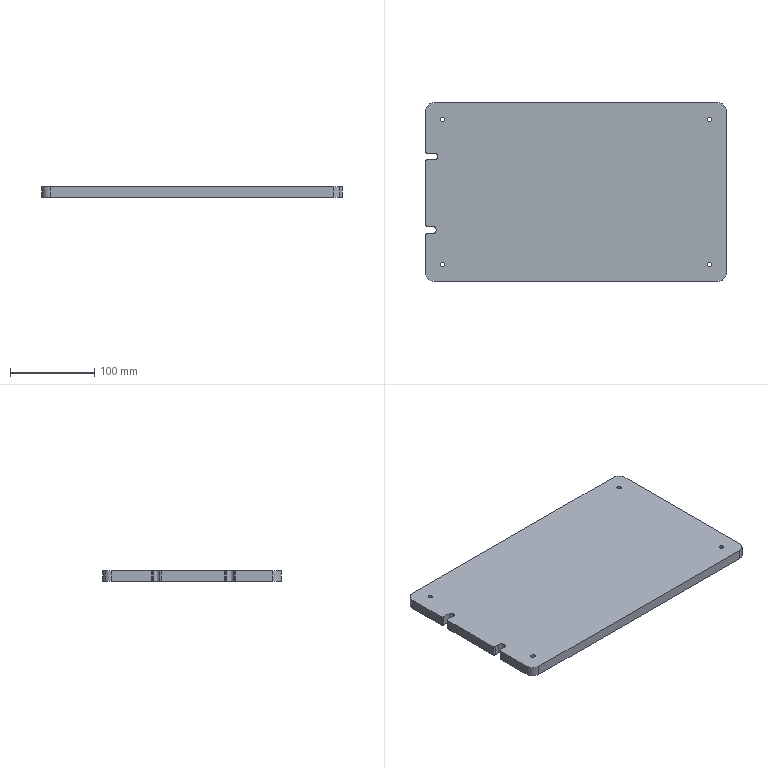Part | STEP file | ASND-0110-6.2aq | 1 solid | 49 faces | box 357.093 x 212.456 x 12 mm | volume 877711 mm3 | cylinder 33 | plane 16 | commonest cylinder face diameters 4 x8 5 x8 30 x8 20 x7 7 x1 9 x1